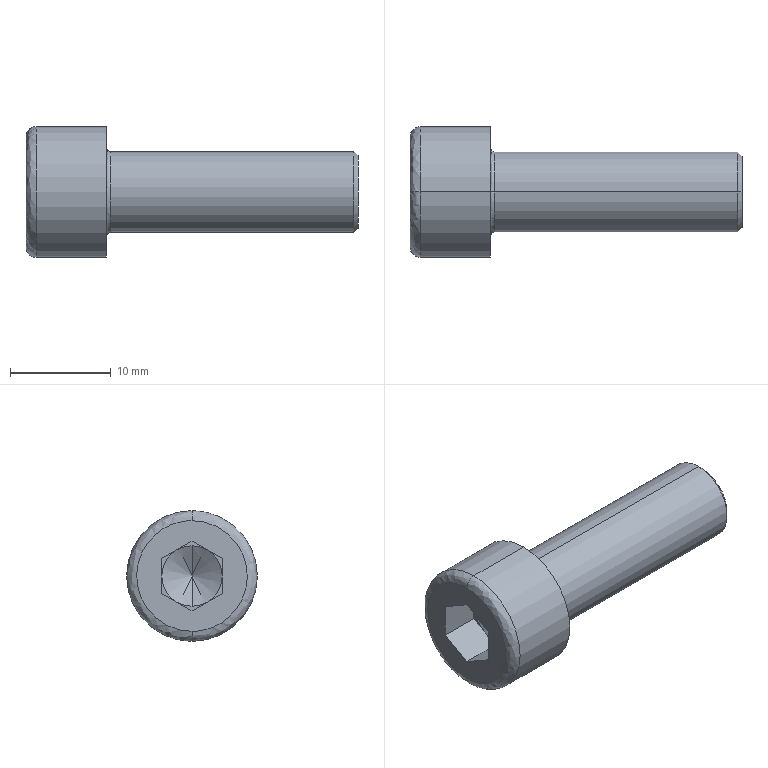Part | SolidWorks | features BaseBody 1 | 1 solid | 27 faces | box 33 x 13 x 13 mm | volume 2168 mm3 | plane 15 | spline 4 | cylinder 4 | cone 4 | commonest cylinder face diameters 8 x2 13 x2
STEP:
#1=CARTESIAN_POINT('',(8.,0.,4.4));
#2=VERTEX_POINT('',#1);
#3=CARTESIAN_POINT('',(8.,0.,-4.4));
#4=VERTEX_POINT('',#3);
#5=CARTESIAN_POINT('',(8.,0.,4.4));
#6=CARTESIAN_POINT('',(8.,0.2797,4.4));
#7=CARTESIAN_POINT('',(8.,0.6919,4.361));
#8=CARTESIAN_POINT('',(8.,1.16,4.249));
#9=CARTESIAN_POINT('',(8.,1.391,4.176));
#10=CARTESIAN_POINT('',(8.,1.489,4.141));
#11=CARTESIAN_POINT('',(8.,1.554,4.116));
#12=CARTESIAN_POINT('',(8.,1.585,4.105));
#13=CARTESIAN_POINT('',(8.,1.758,4.036));
#14=CARTESIAN_POINT('',(8.,1.96,3.944));
#15=CARTESIAN_POINT('',(8.,2.154,3.837));
#16=CARTESIAN_POINT('',(8.,2.282,3.763));
#17=CARTESIAN_POINT('',(8.,2.344,3.724));
#18=CARTESIAN_POINT('',(8.,2.662,3.517));
#19=CARTESIAN_POINT('',(8.,2.897,3.326));
#20=CARTESIAN_POINT('',(8.,3.219,3.004));
#21=CARTESIAN_POINT('',(8.,3.37,2.836));
#22=CARTESIAN_POINT('',(8.,3.509,2.656));
#23=CARTESIAN_POINT('',(8.,3.598,2.534));
#24=CARTESIAN_POINT('',(8.,3.642,2.47));
#25=CARTESIAN_POINT('',(8.,3.764,2.283));
#26=CARTESIAN_POINT('',(8.,3.876,2.092));
#27=CARTESIAN_POINT('',(8.,3.989,1.859));
#28=CARTESIAN_POINT('',(8.,4.042,1.74));
#29=CARTESIAN_POINT('',(8.,4.063,1.689));
#30=CARTESIAN_POINT('',(8.,4.077,1.654));
#31=CARTESIAN_POINT('',(8.,4.085,1.636));
#32=CARTESIAN_POINT('',(8.,4.297,1.1));
#33=CARTESIAN_POINT('',(8.,4.4,0.5592));
#34=CARTESIAN_POINT('',(8.,4.4,-0.2796));
#35=CARTESIAN_POINT('',(8.,4.361,-0.6917));
#36=CARTESIAN_POINT('',(8.,4.249,-1.16));
#37=CARTESIAN_POINT('',(8.,4.176,-1.391));
#38=CARTESIAN_POINT('',(8.,4.141,-1.489));
#39=CARTESIAN_POINT('',(8.,4.116,-1.554));
#40=CARTESIAN_POINT('',(8.,4.105,-1.585));
#41=CARTESIAN_POINT('',(8.,4.036,-1.758));
#42=CARTESIAN_POINT('',(8.,3.944,-1.96));
#43=CARTESIAN_POINT('',(8.,3.837,-2.154));
#44=CARTESIAN_POINT('',(8.,3.763,-2.282));
#45=CARTESIAN_POINT('',(8.,3.724,-2.344));
#46=CARTESIAN_POINT('',(8.,3.517,-2.662));
#47=CARTESIAN_POINT('',(8.,3.326,-2.897));
#48=CARTESIAN_POINT('',(8.,3.004,-3.219));
#49=CARTESIAN_POINT('',(8.,2.836,-3.37));
#50=CARTESIAN_POINT('',(8.,2.656,-3.509));
#51=CARTESIAN_POINT('',(8.,2.534,-3.598));
#52=CARTESIAN_POINT('',(8.,2.47,-3.642));
#53=CARTESIAN_POINT('',(8.,2.283,-3.764));
#54=CARTESIAN_POINT('',(8.,2.092,-3.876));
#55=CARTESIAN_POINT('',(8.,1.859,-3.989));
#56=CARTESIAN_POINT('',(8.,1.74,-4.042));
#57=CARTESIAN_POINT('',(8.,1.689,-4.063));
#58=CARTESIAN_POINT('',(8.,1.654,-4.077));
#59=CARTESIAN_POINT('',(8.,1.636,-4.085));
#60=CARTESIAN_POINT('',(8.,1.1,-4.297));
#61=CARTESIAN_POINT('',(8.,0.5597,-4.4));
#62=CARTESIAN_POINT('',(8.,0.,-4.4));
#63=B_SPLINE_CURVE_WITH_KNOTS('',3,(#5,#6,#7,#8,#9,#10,#11,#12,#13,#14,#15,#16,#17,#18,#19,#20,#21,#22,#23,#24,#25,#26,#27,#28,#29,#30,#31,#32,#33,#34,#35,#36,#37,#38,#39,#40,#41,#42,#43,#44,#45,#46,#47,#48,#49,#50,#51,#52,#53,#54,#55,#56,#57,#58,#59,#60,#61,#62),.UNSPECIFIED.,.F.,.F.,(4,1,1,1,2,2,1,2,2,2,1,2,2,1,1,1,2,2,2,1,1,1,2,2,1,2,2,2,1,2,2,1,1,1,2,2,4),(0.,0.0625,0.09375,0.1094,0.1172,0.125,0.1562,0.1719,0.1875,0.25,0.2812,0.2969,0.3125,0.3437,0.3594,0.3672,0.3711,0.375,0.5,0.5625,0.5937,0.6094,0.6172,0.625,0.6562,0.6719,0.6875,0.75,0.7812,0.7969,0.8125,0.8437,0.8594,0.8672,0.8711,0.875,1.),.UNSPECIFIED.);
#64=EDGE_CURVE('',#2,#4,#63,.T.);
#65=ORIENTED_EDGE('',*,*,#64,.F.);
#66=CARTESIAN_POINT('',(8.4,0.,4.));
#67=VERTEX_POINT('',#66);
#68=CARTESIAN_POINT('',(8.4,0.,4.4));
#69=DIRECTION('',(0.,-1.,0.));
#70=DIRECTION('',(0.,0.,1.));
#71=AXIS2_PLACEMENT_3D('',#68,#69,#70);
#72=CIRCLE('',#71,0.4);
#73=EDGE_CURVE('',#2,#67,#72,.T.);
#74=ORIENTED_EDGE('',*,*,#73,.T.);
#75=CARTESIAN_POINT('',(8.4,0.,-4.));
#76=VERTEX_POINT('',#75);
#77=CARTESIAN_POINT('',(8.4,0.,0.));
#78=DIRECTION('',(1.,0.,0.));
#79=DIRECTION('',(0.,0.,1.));
#80=AXIS2_PLACEMENT_3D('',#77,#78,#79);
#81=CIRCLE('',#80,4.);
#82=EDGE_CURVE('',#76,#67,#81,.T.);
#83=ORIENTED_EDGE('',*,*,#82,.F.);
#84=CARTESIAN_POINT('',(8.4,0.,-4.4));
#85=DIRECTION('',(0.,1.,0.));
#86=DIRECTION('',(0.,0.,-1.));
#87=AXIS2_PLACEMENT_3D('',#84,#85,#86);
#88=CIRCLE('',#87,0.4);
#89=EDGE_CURVE('',#4,#76,#88,.T.);
#90=ORIENTED_EDGE('',*,*,#89,.F.);
#91=EDGE_LOOP('',(#65,#74,#83,#90));
#92=FACE_OUTER_BOUND('',#91,.T.);
#93=CARTESIAN_POINT('',(8.,0.,-4.4));
#94=CARTESIAN_POINT('',(8.,8.8,-4.4));
#95=CARTESIAN_POINT('',(8.,8.8,4.4));
#96=CARTESIAN_POINT('',(8.,0.,4.4));
#97=CARTESIAN_POINT('',(8.,0.,-4.166));
#98=CARTESIAN_POINT('',(8.,8.331,-4.166));
#99=CARTESIAN_POINT('',(8.,8.331,4.166));
#100=CARTESIAN_POINT('',(8.,0.,4.166));
#101=CARTESIAN_POINT('',(8.166,0.,-4.));
#102=CARTESIAN_POINT('',(8.166,8.,-4.));
#103=CARTESIAN_POINT('',(8.166,8.,4.));
#104=CARTESIAN_POINT('',(8.166,0.,4.));
#105=CARTESIAN_POINT('',(8.4,0.,-4.));
#106=CARTESIAN_POINT('',(8.4,8.,-4.));
#107=CARTESIAN_POINT('',(8.4,8.,4.));
#108=CARTESIAN_POINT('',(8.4,0.,4.));
#109=(BOUNDED_SURFACE()B_SPLINE_SURFACE(3,3,((#93,#94,#95,#96),(#97,#98,#99,#100),(#101,#102,#103,#104),(#105,#106,#107,#108)),.UNSPECIFIED.,.F.,.F.,.T.)B_SPLINE_SURFACE_WITH_KNOTS((4,4),(4,4),(0.,1.),(0.,1.),.UNSPECIFIED.)GEOMETRIC_REPRESENTATION_ITEM()RATIONAL_B_SPLINE_SURFACE(((1.,0.3333,0.3333,1.),(0.8047,0.2682,0.2682,0.8047),(0.8047,0.2682,0.2682,0.8047),(1.,0.3333,0.3333,1.)))REPRESENTATION_ITEM('')SURFACE());
#110=ADVANCED_FACE('',(#92),#109,.F.);
#111=CARTESIAN_POINT('',(1.,0.,6.5));
#112=VERTEX_POINT('',#111);
#113=CARTESIAN_POINT('',(1.,0.,-6.5));
#114=VERTEX_POINT('',#113);
#115=CARTESIAN_POINT('',(1.,0.,0.));
#116=DIRECTION('',(1.,0.,0.));
#117=DIRECTION('',(0.,0.,1.));
#118=AXIS2_PLACEMENT_3D('',#115,#116,#117);
#119=CIRCLE('',#118,6.5);
#120=EDGE_CURVE('',#112,#114,#119,.T.);
#121=ORIENTED_EDGE('',*,*,#120,.F.);
#122=CARTESIAN_POINT('',(0.,0.,5.5));
#123=VERTEX_POINT('',#122);
#124=CARTESIAN_POINT('',(1.,0.,5.5));
#125=DIRECTION('',(0.,-1.,0.));
#126=DIRECTION('',(0.,0.,1.));
#127=AXIS2_PLACEMENT_3D('',#124,#125,#126);
#128=CIRCLE('',#127,1.);
#129=EDGE_CURVE('',#112,#123,#128,.T.);
#130=ORIENTED_EDGE('',*,*,#129,.T.);
#131=CARTESIAN_POINT('',(0.,0.,-5.5));
#132=VERTEX_POINT('',#131);
#133=CARTESIAN_POINT('',(0.,0.,5.5));
#134=CARTESIAN_POINT('',(0.,-11.,5.5));
#135=CARTESIAN_POINT('',(0.,-11.,-5.5));
#136=CARTESIAN_POINT('',(0.,0.,-5.5));
#137=(BOUNDED_CURVE()B_SPLINE_CURVE(3,(#133,#134,#135,#136),.UNSPECIFIED.,.F.,.F.)B_SPLINE_CURVE_WITH_KNOTS((4,4),(0.,1.),.UNSPECIFIED.)CURVE()GEOMETRIC_REPRESENTATION_ITEM()RATIONAL_B_SPLINE_CURVE((1.,0.3333,0.3333,1.))REPRESENTATION_ITEM(''));
#138=EDGE_CURVE('',#123,#132,#137,.T.);
#139=ORIENTED_EDGE('',*,*,#138,.T.);
#140=CARTESIAN_POINT('',(1.,0.,-5.5));
#141=DIRECTION('',(0.,1.,0.));
#142=DIRECTION('',(0.,0.,-1.));
#143=AXIS2_PLACEMENT_3D('',#140,#141,#142);
#144=CIRCLE('',#143,1.);
#145=EDGE_CURVE('',#114,#132,#144,.T.);
#146=ORIENTED_EDGE('',*,*,#145,.F.);
#147=EDGE_LOOP('',(#121,#130,#139,#146));
#148=FACE_OUTER_BOUND('',#147,.T.);
#149=CARTESIAN_POINT('',(1.,0.,6.5));
#150=CARTESIAN_POINT('',(1.,-13.,6.5));
#151=CARTESIAN_POINT('',(1.,-13.,-6.5));
#152=CARTESIAN_POINT('',(1.,0.,-6.5));
#153=CARTESIAN_POINT('',(0.4142,0.,6.5));
#154=CARTESIAN_POINT('',(0.4142,-13.,6.5));
#155=CARTESIAN_POINT('',(0.4142,-13.,-6.5));
#156=CARTESIAN_POINT('',(0.4142,0.,-6.5));
#157=CARTESIAN_POINT('',(0.,0.,6.086));
#158=CARTESIAN_POINT('',(0.,-12.172,6.086));
#159=CARTESIAN_POINT('',(0.,-12.172,-6.086));
#160=CARTESIAN_POINT('',(0.,0.,-6.086));
#161=CARTESIAN_POINT('',(0.,0.,5.5));
#162=CARTESIAN_POINT('',(0.,-11.,5.5));
#163=CARTESIAN_POINT('',(0.,-11.,-5.5));
#164=CARTESIAN_POINT('',(0.,0.,-5.5));
#165=(BOUNDED_SURFACE()B_SPLINE_SURFACE(3,3,((#149,#150,#151,#152),(#153,#154,#155,#156),(#157,#158,#159,#160),(#161,#162,#163,#164)),.UNSPECIFIED.,.F.,.F.,.T.)B_SPLINE_SURFACE_WITH_KNOTS((4,4),(4,4),(0.,1.),(0.,1.),.UNSPECIFIED.)GEOMETRIC_REPRESENTATION_ITEM()RATIONAL_B_SPLINE_SURFACE(((1.,0.3333,0.3333,1.),(0.8047,0.2682,0.2682,0.8047),(0.8047,0.2682,0.2682,0.8047),(1.,0.3333,0.3333,1.)))REPRESENTATION_ITEM('')SURFACE());
#166=ADVANCED_FACE('',(#148),#165,.T.);
#167=CARTESIAN_POINT('',(32.6,0.,4.));
#168=VERTEX_POINT('',#167);
#169=CARTESIAN_POINT('',(32.6,0.,-4.));
#170=VERTEX_POINT('',#169);
#171=CARTESIAN_POINT('',(32.6,0.,0.));
#172=DIRECTION('',(-1.,0.,0.));
#173=DIRECTION('',(0.,0.,1.));
#174=AXIS2_PLACEMENT_3D('',#171,#172,#173);
#175=CIRCLE('',#174,4.);
#176=EDGE_CURVE('',#168,#170,#175,.T.);
#177=ORIENTED_EDGE('',*,*,#176,.T.);
#178=CARTESIAN_POINT('',(33.,0.,-4.));
#179=DIRECTION('',(-1.,0.,0.));
#180=VECTOR('',#179,1000.);
#181=LINE('',#178,#180);
#182=EDGE_CURVE('',#170,#76,#181,.T.);
#183=ORIENTED_EDGE('',*,*,#182,.T.);
#184=ORIENTED_EDGE('',*,*,#82,.T.);
#185=CARTESIAN_POINT('',(33.,0.,4.));
#186=DIRECTION('',(-1.,0.,0.));
#187=VECTOR('',#186,1000.);
#188=LINE('',#185,#187);
#189=EDGE_CURVE('',#168,#67,#188,.T.);
#190=ORIENTED_EDGE('',*,*,#189,.F.);
#191=EDGE_LOOP('',(#177,#183,#184,#190));
#192=FACE_OUTER_BOUND('',#191,.T.);
#193=CARTESIAN_POINT('',(33.,0.,0.));
#194=DIRECTION('',(-1.,0.,0.));
#195=DIRECTION('',(0.,0.,1.));
#196=AXIS2_PLACEMENT_3D('',#193,#194,#195);
#197=CYLINDRICAL_SURFACE('',#196,4.);
#198=ADVANCED_FACE('',(#192),#197,.T.);
#199=CARTESIAN_POINT('',(33.,0.,3.6));
#200=VERTEX_POINT('',#199);
#201=CARTESIAN_POINT('',(33.,0.,-3.6));
#202=VERTEX_POINT('',#201);
#203=CARTESIAN_POINT('',(33.,0.,0.));
#204=DIRECTION('',(-1.,0.,0.));
#205=DIRECTION('',(0.,0.,1.));
#206=AXIS2_PLACEMENT_3D('',#203,#204,#205);
#207=CIRCLE('',#206,3.6);
#208=EDGE_CURVE('',#200,#202,#207,.T.);
#209=ORIENTED_EDGE('',*,*,#208,.T.);
#210=CARTESIAN_POINT('',(32.6,0.,-4.));
#211=DIRECTION('',(-0.7071,0.,-0.7071));
#212=VECTOR('',#211,1000.);
#213=LINE('',#210,#212);
#214=EDGE_CURVE('',#202,#170,#213,.T.);
#215=ORIENTED_EDGE('',*,*,#214,.T.);
#216=ORIENTED_EDGE('',*,*,#176,.F.);
#217=CARTESIAN_POINT('',(32.6,0.,4.));
#218=DIRECTION('',(-0.7071,0.,0.7071));
#219=VECTOR('',#218,1000.);
#220=LINE('',#217,#219);
#221=EDGE_CURVE('',#200,#168,#220,.T.);
#222=ORIENTED_EDGE('',*,*,#221,.F.);
#223=EDGE_LOOP('',(#209,#215,#216,#222));
#224=FACE_OUTER_BOUND('',#223,.T.);
#225=CARTESIAN_POINT('',(32.6,0.,0.));
#226=DIRECTION('',(-1.,0.,0.));
#227=DIRECTION('',(0.,0.,1.));
#228=AXIS2_PLACEMENT_3D('',#225,#226,#227);
#229=CONICAL_SURFACE('',#228,4.,0.7854);
#230=ADVANCED_FACE('',(#224),#229,.T.);
#231=CARTESIAN_POINT('',(8.,0.,-6.5));
#232=VERTEX_POINT('',#231);
#233=CARTESIAN_POINT('',(8.,0.,6.5));
#234=VERTEX_POINT('',#233);
#235=CARTESIAN_POINT('',(8.,0.,0.));
#236=DIRECTION('',(1.,0.,0.));
#237=DIRECTION('',(0.,0.,1.));
#238=AXIS2_PLACEMENT_3D('',#235,#236,#237);
#239=CIRCLE('',#238,6.5);
#240=EDGE_CURVE('',#232,#234,#239,.T.);
#241=ORIENTED_EDGE('',*,*,#240,.F.);
#242=CARTESIAN_POINT('',(8.,0.,-6.5));
#243=DIRECTION('',(-1.,0.,0.));
#244=VECTOR('',#243,1000.);
#245=LINE('',#242,#244);
#246=EDGE_CURVE('',#232,#114,#245,.T.);
#247=ORIENTED_EDGE('',*,*,#246,.T.);
#248=CARTESIAN_POINT('',(1.,0.,0.));
#249=DIRECTION('',(1.,0.,0.));
#250=DIRECTION('',(0.,0.,1.));
#251=AXIS2_PLACEMENT_3D('',#248,#249,#250);
#252=CIRCLE('',#251,6.5);
#253=EDGE_CURVE('',#114,#112,#252,.T.);
#254=ORIENTED_EDGE('',*,*,#253,.T.);
#255=CARTESIAN_POINT('',(8.,0.,6.5));
#256=DIRECTION('',(-1.,0.,0.));
#257=VECTOR('',#256,1000.);
#258=LINE('',#255,#257);
#259=EDGE_CURVE('',#234,#112,#258,.T.);
#260=ORIENTED_EDGE('',*,*,#259,.F.);
#261=EDGE_LOOP('',(#241,#247,#254,#260));
#262=FACE_OUTER_BOUND('',#261,.T.);
#263=CARTESIAN_POINT('',(8.,0.,0.));
#264=DIRECTION('',(-1.,0.,0.));
#265=DIRECTION('',(0.,0.,1.));
#266=AXIS2_PLACEMENT_3D('',#263,#264,#265);
#267=CYLINDRICAL_SURFACE('',#266,6.5);
#268=ADVANCED_FACE('',(#262),#267,.T.);
#269=CARTESIAN_POINT('',(5.732,0.,0.));
#270=VERTEX_POINT('',#269);
#271=CARTESIAN_POINT('',(4.,0.,3.));
#272=VERTEX_POINT('',#271);
#273=CARTESIAN_POINT('',(4.,0.,3.));
#274=DIRECTION('',(-0.5,0.,0.866));
#275=VECTOR('',#274,1000.);
#276=LINE('',#273,#275);
#277=EDGE_CURVE('',#270,#272,#276,.T.);
#278=ORIENTED_EDGE('',*,*,#277,.F.);
#279=CARTESIAN_POINT('',(4.,0.,-3.));
#280=VERTEX_POINT('',#279);
#281=CARTESIAN_POINT('',(4.,0.,-3.));
#282=DIRECTION('',(-0.5,0.,-0.866));
#283=VECTOR('',#282,1000.);
#284=LINE('',#281,#283);
#285=EDGE_CURVE('',#270,#280,#284,.T.);
#286=ORIENTED_EDGE('',*,*,#285,.T.);
#287=CARTESIAN_POINT('',(4.,-1.5,-2.598));
#288=VERTEX_POINT('',#287);
#289=CARTESIAN_POINT('',(4.,0.,0.));
#290=DIRECTION('',(1.,0.,0.));
#291=DIRECTION('',(0.,0.,1.));
#292=AXIS2_PLACEMENT_3D('',#289,#290,#291);
#293=CIRCLE('',#292,3.);
#294=EDGE_CURVE('',#288,#280,#293,.T.);
#295=ORIENTED_EDGE('',*,*,#294,.F.);
#296=CARTESIAN_POINT('',(4.,-3.,0.));
#297=VERTEX_POINT('',#296);
#298=CARTESIAN_POINT('',(4.,0.,0.));
#299=DIRECTION('',(-1.,0.,0.));
#300=DIRECTION('',(0.,0.,1.));
#301=AXIS2_PLACEMENT_3D('',#298,#299,#300);
#302=CIRCLE('',#301,3.);
#303=EDGE_CURVE('',#288,#297,#302,.T.);
#304=ORIENTED_EDGE('',*,*,#303,.T.);
#305=CARTESIAN_POINT('',(4.,-1.5,2.598));
#306=VERTEX_POINT('',#305);
#307=CARTESIAN_POINT('',(4.,0.,0.));
#308=DIRECTION('',(1.,0.,0.));
#309=DIRECTION('',(0.,0.,1.));
#310=AXIS2_PLACEMENT_3D('',#307,#308,#309);
#311=CIRCLE('',#310,3.);
#312=EDGE_CURVE('',#306,#297,#311,.T.);
#313=ORIENTED_EDGE('',*,*,#312,.F.);
#314=CARTESIAN_POINT('',(4.,0.,0.));
#315=DIRECTION('',(1.,0.,0.));
#316=DIRECTION('',(0.,0.,1.));
#317=AXIS2_PLACEMENT_3D('',#314,#315,#316);
#318=CIRCLE('',#317,3.);
#319=EDGE_CURVE('',#272,#306,#318,.T.);
#320=ORIENTED_EDGE('',*,*,#319,.F.);
#321=EDGE_LOOP('',(#278,#286,#295,#304,#313,#320));
#322=FACE_OUTER_BOUND('',#321,.T.);
#323=CARTESIAN_POINT('',(4.,0.,0.));
#324=DIRECTION('',(-1.,0.,0.));
#325=DIRECTION('',(0.,0.,1.));
#326=AXIS2_PLACEMENT_3D('',#323,#324,#325);
#327=CONICAL_SURFACE('',#326,3.,1.047);
#328=ADVANCED_FACE('',(#322),#327,.F.);
#329=ORIENTED_EDGE('',*,*,#182,.F.);
#330=CARTESIAN_POINT('',(32.6,0.,0.));
#331=DIRECTION('',(-1.,0.,0.));
#332=DIRECTION('',(0.,0.,1.));
#333=AXIS2_PLACEMENT_3D('',#330,#331,#332);
#334=CIRCLE('',#333,4.);
#335=EDGE_CURVE('',#170,#168,#334,.T.);
#336=ORIENTED_EDGE('',*,*,#335,.T.);
#337=ORIENTED_EDGE('',*,*,#189,.T.);
#338=CARTESIAN_POINT('',(8.4,0.,0.));
#339=DIRECTION('',(1.,0.,0.));
#340=DIRECTION('',(0.,0.,1.));
#341=AXIS2_PLACEMENT_3D('',#338,#339,#340);
#342=CIRCLE('',#341,4.);
#343=EDGE_CURVE('',#67,#76,#342,.T.);
#344=ORIENTED_EDGE('',*,*,#343,.T.);
#345=EDGE_LOOP('',(#329,#336,#337,#344));
#346=FACE_OUTER_BOUND('',#345,.T.);
#347=CARTESIAN_POINT('',(33.,0.,0.));
#348=DIRECTION('',(-1.,0.,0.));
#349=DIRECTION('',(0.,0.,1.));
#350=AXIS2_PLACEMENT_3D('',#347,#348,#349);
#351=CYLINDRICAL_SURFACE('',#350,4.);
#352=ADVANCED_FACE('',(#346),#351,.T.);
#353=ORIENTED_EDGE('',*,*,#73,.F.);
#354=CARTESIAN_POINT('',(8.,0.,-4.4));
#355=CARTESIAN_POINT('',(8.,-0.2797,-4.4));
#356=CARTESIAN_POINT('',(8.,-0.6919,-4.361));
#357=CARTESIAN_POINT('',(8.,-1.16,-4.249));
#358=CARTESIAN_POINT('',(8.,-1.391,-4.176));
#359=CARTESIAN_POINT('',(8.,-1.489,-4.141));
#360=CARTESIAN_POINT('',(8.,-1.554,-4.116));
#361=CARTESIAN_POINT('',(8.,-1.585,-4.105));
#362=CARTESIAN_POINT('',(8.,-1.758,-4.036));
#363=CARTESIAN_POINT('',(8.,-1.96,-3.944));
#364=CARTESIAN_POINT('',(8.,-2.154,-3.837));
#365=CARTESIAN_POINT('',(8.,-2.282,-3.763));
#366=CARTESIAN_POINT('',(8.,-2.344,-3.724));
#367=CARTESIAN_POINT('',(8.,-2.662,-3.517));
#368=CARTESIAN_POINT('',(8.,-2.897,-3.326));
#369=CARTESIAN_POINT('',(8.,-3.219,-3.004));
#370=CARTESIAN_POINT('',(8.,-3.37,-2.836));
#371=CARTESIAN_POINT('',(8.,-3.509,-2.656));
#372=CARTESIAN_POINT('',(8.,-3.598,-2.534));
#373=CARTESIAN_POINT('',(8.,-3.642,-2.47));
#374=CARTESIAN_POINT('',(8.,-3.764,-2.283));
#375=CARTESIAN_POINT('',(8.,-3.876,-2.092));
#376=CARTESIAN_POINT('',(8.,-3.989,-1.859));
#377=CARTESIAN_POINT('',(8.,-4.042,-1.74));
#378=CARTESIAN_POINT('',(8.,-4.063,-1.689));
#379=CARTESIAN_POINT('',(8.,-4.077,-1.654));
#380=CARTESIAN_POINT('',(8.,-4.085,-1.636));
#381=CARTESIAN_POINT('',(8.,-4.297,-1.1));
#382=CARTESIAN_POINT('',(8.,-4.4,-0.5592));
#383=CARTESIAN_POINT('',(8.,-4.4,0.2796));
#384=CARTESIAN_POINT('',(8.,-4.361,0.6917));
#385=CARTESIAN_POINT('',(8.,-4.249,1.16));
#386=CARTESIAN_POINT('',(8.,-4.176,1.391));
#387=CARTESIAN_POINT('',(8.,-4.141,1.489));
#388=CARTESIAN_POINT('',(8.,-4.116,1.554));
#389=CARTESIAN_POINT('',(8.,-4.105,1.585));
#390=CARTESIAN_POINT('',(8.,-4.036,1.758));
#391=CARTESIAN_POINT('',(8.,-3.944,1.96));
#392=CARTESIAN_POINT('',(8.,-3.837,2.154));
#393=CARTESIAN_POINT('',(8.,-3.763,2.282));
#394=CARTESIAN_POINT('',(8.,-3.724,2.344));
#395=CARTESIAN_POINT('',(8.,-3.517,2.662));
#396=CARTESIAN_POINT('',(8.,-3.326,2.897));
#397=CARTESIAN_POINT('',(8.,-3.004,3.219));
#398=CARTESIAN_POINT('',(8.,-2.836,3.37));
#399=CARTESIAN_POINT('',(8.,-2.656,3.509));
#400=CARTESIAN_POINT('',(8.,-2.534,3.598));
#401=CARTESIAN_POINT('',(8.,-2.47,3.642));
#402=CARTESIAN_POINT('',(8.,-2.283,3.764));
#403=CARTESIAN_POINT('',(8.,-2.092,3.876));
#404=CARTESIAN_POINT('',(8.,-1.859,3.989));
#405=CARTESIAN_POINT('',(8.,-1.74,4.042));
#406=CARTESIAN_POINT('',(8.,-1.689,4.063));
#407=CARTESIAN_POINT('',(8.,-1.654,4.077));
#408=CARTESIAN_POINT('',(8.,-1.636,4.085));
#409=CARTESIAN_POINT('',(8.,-1.1,4.297));
#410=CARTESIAN_POINT('',(8.,-0.5597,4.4));
#411=CARTESIAN_POINT('',(8.,0.,4.4));
#412=B_SPLINE_CURVE_WITH_KNOTS('',3,(#354,#355,#356,#357,#358,#359,#360,#361,#362,#363,#364,#365,#366,#367,#368,#369,#370,#371,#372,#373,#374,#375,#376,#377,#378,#379,#380,#381,#382,#383,#384,#385,#386,#387,#388,#389,#390,#391,#392,#393,#394,#395,#396,#397,#398,#399,#400,#401,#402,#403,#404,#405,#406,#407,#408,#409,#410,#411),.UNSPECIFIED.,.F.,.F.,(4,1,1,1,2,2,1,2,2,2,1,2,2,1,1,1,2,2,2,1,1,1,2,2,1,2,2,2,1,2,2,1,1,1,2,2,4),(0.,0.0625,0.09375,0.1094,0.1172,0.125,0.1563,0.1719,0.1875,0.25,0.2813,0.2969,0.3125,0.3438,0.3594,0.3672,0.3711,0.375,0.5,0.5625,0.5938,0.6094,0.6172,0.625,0.6563,0.6719,0.6875,0.75,0.7813,0.7969,0.8125,0.8438,0.8594,0.8672,0.8711,0.875,1.),.UNSPECIFIED.);
#413=EDGE_CURVE('',#4,#2,#412,.T.);
#414=ORIENTED_EDGE('',*,*,#413,.F.);
#415=ORIENTED_EDGE('',*,*,#89,.T.);
#416=ORIENTED_EDGE('',*,*,#343,.F.);
#417=EDGE_LOOP('',(#353,#414,#415,#416));
#418=FACE_OUTER_BOUND('',#417,.T.);
#419=CARTESIAN_POINT('',(8.,0.,4.4));
#420=CARTESIAN_POINT('',(8.,-8.8,4.4));
#421=CARTESIAN_POINT('',(8.,-8.8,-4.4));
#422=CARTESIAN_POINT('',(8.,0.,-4.4));
#423=CARTESIAN_POINT('',(8.,0.,4.166));
#424=CARTESIAN_POINT('',(8.,-8.331,4.166));
#425=CARTESIAN_POINT('',(8.,-8.331,-4.166));
#426=CARTESIAN_POINT('',(8.,0.,-4.166));
#427=CARTESIAN_POINT('',(8.166,0.,4.));
#428=CARTESIAN_POINT('',(8.166,-8.,4.));
#429=CARTESIAN_POINT('',(8.166,-8.,-4.));
#430=CARTESIAN_POINT('',(8.166,0.,-4.));
#431=CARTESIAN_POINT('',(8.4,0.,4.));
#432=CARTESIAN_POINT('',(8.4,-8.,4.));
#433=CARTESIAN_POINT('',(8.4,-8.,-4.));
#434=CARTESIAN_POINT('',(8.4,0.,-4.));
#435=(BOUNDED_SURFACE()B_SPLINE_SURFACE(3,3,((#419,#420,#421,#422),(#423,#424,#425,#426),(#427,#428,#429,#430),(#431,#432,#433,#434)),.UNSPECIFIED.,.F.,.F.,.F.)B_SPLINE_SURFACE_WITH_KNOTS((4,4),(4,4),(0.,1.),(0.,1.),.UNSPECIFIED.)GEOMETRIC_REPRESENTATION_ITEM()RATIONAL_B_SPLINE_SURFACE(((1.,0.3333,0.3333,1.),(0.8047,0.2682,0.2682,0.8047),(0.8047,0.2682,0.2682,0.8047),(1.,0.3333,0.3333,1.)))REPRESENTATION_ITEM('')SURFACE());
#436=ADVANCED_FACE('',(#418),#435,.F.);
#437=ORIENTED_EDGE('',*,*,#214,.F.);
#438=CARTESIAN_POINT('',(33.,0.,0.));
#439=DIRECTION('',(-1.,0.,0.));
#440=DIRECTION('',(0.,0.,1.));
#441=AXIS2_PLACEMENT_3D('',#438,#439,#440);
#442=CIRCLE('',#441,3.6);
#443=EDGE_CURVE('',#202,#200,#442,.T.);
#444=ORIENTED_EDGE('',*,*,#443,.T.);
#445=ORIENTED_EDGE('',*,*,#221,.T.);
#446=ORIENTED_EDGE('',*,*,#335,.F.);
#447=EDGE_LOOP('',(#437,#444,#445,#446));
#448=FACE_OUTER_BOUND('',#447,.T.);
#449=CARTESIAN_POINT('',(32.6,0.,0.));
#450=DIRECTION('',(-1.,0.,0.));
#451=DIRECTION('',(0.,0.,1.));
#452=AXIS2_PLACEMENT_3D('',#449,#450,#451);
#453=CONICAL_SURFACE('',#452,4.,0.7854);
#454=ADVANCED_FACE('',(#448),#453,.T.);
#455=CARTESIAN_POINT('',(8.,0.,0.));
#456=DIRECTION('',(1.,0.,0.));
#457=DIRECTION('',(0.,0.,1.));
#458=AXIS2_PLACEMENT_3D('',#455,#456,#457);
#459=CIRCLE('',#458,6.5);
#460=EDGE_CURVE('',#234,#232,#459,.T.);
#461=ORIENTED_EDGE('',*,*,#460,.T.);
#462=ORIENTED_EDGE('',*,*,#240,.T.);
#463=EDGE_LOOP('',(#461,#462));
#464=FACE_OUTER_BOUND('',#463,.T.);
#465=ORIENTED_EDGE('',*,*,#413,.T.);
#466=ORIENTED_EDGE('',*,*,#64,.T.);
#467=EDGE_LOOP('',(#465,#466));
#468=FACE_BOUND('',#467,.T.);
#469=CARTESIAN_POINT('',(8.,0.,0.));
#470=DIRECTION('',(1.,0.,0.));
#471=DIRECTION('',(0.,0.,-1.));
#472=AXIS2_PLACEMENT_3D('',#469,#470,#471);
#473=PLANE('',#472);
#474=ADVANCED_FACE('',(#464,#468),#473,.T.);
#475=ORIENTED_EDGE('',*,*,#208,.F.);
#476=ORIENTED_EDGE('',*,*,#443,.F.);
#477=EDGE_LOOP('',(#475,#476));
#478=FACE_OUTER_BOUND('',#477,.T.);
#479=CARTESIAN_POINT('',(33.,0.,0.));
#480=DIRECTION('',(1.,0.,0.));
#481=DIRECTION('',(0.,0.,-1.));
#482=AXIS2_PLACEMENT_3D('',#479,#480,#481);
#483=PLANE('',#482);
#484=ADVANCED_FACE('',(#478),#483,.T.);
#485=ORIENTED_EDGE('',*,*,#246,.F.);
#486=ORIENTED_EDGE('',*,*,#460,.F.);
#487=ORIENTED_EDGE('',*,*,#259,.T.);
#488=ORIENTED_EDGE('',*,*,#120,.T.);
#489=EDGE_LOOP('',(#485,#486,#487,#488));
#490=FACE_OUTER_BOUND('',#489,.T.);
#491=CARTESIAN_POINT('',(8.,0.,0.));
#492=DIRECTION('',(-1.,0.,0.));
#493=DIRECTION('',(0.,0.,1.));
#494=AXIS2_PLACEMENT_3D('',#491,#492,#493);
#495=CYLINDRICAL_SURFACE('',#494,6.5);
#496=ADVANCED_FACE('',(#490),#495,.T.);
#497=ORIENTED_EDGE('',*,*,#129,.F.);
#498=ORIENTED_EDGE('',*,*,#253,.F.);
#499=ORIENTED_EDGE('',*,*,#145,.T.);
#500=CARTESIAN_POINT('',(0.,0.,-5.5));
#501=CARTESIAN_POINT('',(0.,11.,-5.5));
#502=CARTESIAN_POINT('',(0.,11.,5.5));
#503=CARTESIAN_POINT('',(0.,0.,5.5));
#504=(BOUNDED_CURVE()B_SPLINE_CURVE(3,(#500,#501,#502,#503),.UNSPECIFIED.,.F.,.F.)B_SPLINE_CURVE_WITH_KNOTS((4,4),(0.,1.),.UNSPECIFIED.)CURVE()GEOMETRIC_REPRESENTATION_ITEM()RATIONAL_B_SPLINE_CURVE((1.,0.3333,0.3333,1.))REPRESENTATION_ITEM(''));
#505=EDGE_CURVE('',#132,#123,#504,.T.);
#506=ORIENTED_EDGE('',*,*,#505,.T.);
#507=EDGE_LOOP('',(#497,#498,#499,#506));
#508=FACE_OUTER_BOUND('',#507,.T.);
#509=CARTESIAN_POINT('',(1.,0.,-6.5));
#510=CARTESIAN_POINT('',(1.,13.,-6.5));
#511=CARTESIAN_POINT('',(1.,13.,6.5));
#512=CARTESIAN_POINT('',(1.,0.,6.5));
#513=CARTESIAN_POINT('',(0.4142,0.,-6.5));
#514=CARTESIAN_POINT('',(0.4142,13.,-6.5));
#515=CARTESIAN_POINT('',(0.4142,13.,6.5));
#516=CARTESIAN_POINT('',(0.4142,0.,6.5));
#517=CARTESIAN_POINT('',(0.,0.,-6.086));
#518=CARTESIAN_POINT('',(0.,12.172,-6.086));
#519=CARTESIAN_POINT('',(0.,12.172,6.086));
#520=CARTESIAN_POINT('',(0.,0.,6.086));
#521=CARTESIAN_POINT('',(0.,0.,-5.5));
#522=CARTESIAN_POINT('',(0.,11.,-5.5));
#523=CARTESIAN_POINT('',(0.,11.,5.5));
#524=CARTESIAN_POINT('',(0.,0.,5.5));
#525=(BOUNDED_SURFACE()B_SPLINE_SURFACE(3,3,((#509,#510,#511,#512),(#513,#514,#515,#516),(#517,#518,#519,#520),(#521,#522,#523,#524)),.UNSPECIFIED.,.F.,.F.,.T.)B_SPLINE_SURFACE_WITH_KNOTS((4,4),(4,4),(0.,1.),(0.,1.),.UNSPECIFIED.)GEOMETRIC_REPRESENTATION_ITEM()RATIONAL_B_SPLINE_SURFACE(((1.,0.3333,0.3333,1.),(0.8047,0.2682,0.2682,0.8047),(0.8047,0.2682,0.2682,0.8047),(1.,0.3333,0.3333,1.)))REPRESENTATION_ITEM('')SURFACE());
#526=ADVANCED_FACE('',(#508),#525,.T.);
#527=CARTESIAN_POINT('',(0.,3.,1.732));
#528=VERTEX_POINT('',#527);
#529=CARTESIAN_POINT('',(0.,3.,-1.732));
#530=VERTEX_POINT('',#529);
#531=CARTESIAN_POINT('',(0.,3.,0.));
#532=DIRECTION('',(0.,0.,-1.));
#533=VECTOR('',#532,1000.);
#534=LINE('',#531,#533);
#535=EDGE_CURVE('',#528,#530,#534,.T.);
#536=ORIENTED_EDGE('',*,*,#535,.F.);
#537=CARTESIAN_POINT('',(0.,0.,3.464));
#538=VERTEX_POINT('',#537);
#539=CARTESIAN_POINT('',(0.,0.,3.464));
#540=DIRECTION('',(0.,0.866,-0.5));
#541=VECTOR('',#540,1000.);
#542=LINE('',#539,#541);
#543=EDGE_CURVE('',#538,#528,#542,.T.);
#544=ORIENTED_EDGE('',*,*,#543,.F.);
#545=CARTESIAN_POINT('',(0.,-3.,1.732));
#546=VERTEX_POINT('',#545);
#547=CARTESIAN_POINT('',(0.,-3.,1.732));
#548=DIRECTION('',(0.,0.866,0.5));
#549=VECTOR('',#548,1000.);
#550=LINE('',#547,#549);
#551=EDGE_CURVE('',#546,#538,#550,.T.);
#552=ORIENTED_EDGE('',*,*,#551,.F.);
#553=CARTESIAN_POINT('',(0.,-3.,-1.732));
#554=VERTEX_POINT('',#553);
#555=CARTESIAN_POINT('',(0.,-3.,0.));
#556=DIRECTION('',(0.,0.,1.));
#557=VECTOR('',#556,1000.);
#558=LINE('',#555,#557);
#559=EDGE_CURVE('',#554,#546,#558,.T.);
#560=ORIENTED_EDGE('',*,*,#559,.F.);
#561=CARTESIAN_POINT('',(0.,0.,-3.464));
#562=VERTEX_POINT('',#561);
#563=CARTESIAN_POINT('',(0.,0.,-3.464));
#564=DIRECTION('',(0.,-0.866,0.5));
#565=VECTOR('',#564,1000.);
#566=LINE('',#563,#565);
#567=EDGE_CURVE('',#562,#554,#566,.T.);
#568=ORIENTED_EDGE('',*,*,#567,.F.);
#569=CARTESIAN_POINT('',(0.,3.,-1.732));
#570=DIRECTION('',(0.,-0.866,-0.5));
#571=VECTOR('',#570,1000.);
#572=LINE('',#569,#571);
#573=EDGE_CURVE('',#530,#562,#572,.T.);
#574=ORIENTED_EDGE('',*,*,#573,.F.);
#575=EDGE_LOOP('',(#536,#544,#552,#560,#568,#574));
#576=FACE_BOUND('',#575,.T.);
#577=ORIENTED_EDGE('',*,*,#505,.F.);
#578=ORIENTED_EDGE('',*,*,#138,.F.);
#579=EDGE_LOOP('',(#577,#578));
#580=FACE_OUTER_BOUND('',#579,.T.);
#581=CARTESIAN_POINT('',(0.,0.,0.));
#582=DIRECTION('',(1.,0.,0.));
#583=DIRECTION('',(0.,0.,-1.));
#584=AXIS2_PLACEMENT_3D('',#581,#582,#583);
#585=PLANE('',#584);
#586=ADVANCED_FACE('',(#576,#580),#585,.F.);
#587=CARTESIAN_POINT('',(4.,0.,-3.464));
#588=VERTEX_POINT('',#587);
#589=CARTESIAN_POINT('',(4.,0.,-3.464));
#590=DIRECTION('',(1.,0.,0.));
#591=VECTOR('',#590,1000.);
#592=LINE('',#589,#591);
#593=EDGE_CURVE('',#562,#588,#592,.T.);
#594=ORIENTED_EDGE('',*,*,#593,.T.);
#595=CARTESIAN_POINT('',(4.,1.5,-2.598));
#596=VERTEX_POINT('',#595);
#597=CARTESIAN_POINT('',(4.,0.,-3.464));
#598=DIRECTION('',(0.,0.866,0.5));
#599=VECTOR('',#598,1000.);
#600=LINE('',#597,#599);
#601=EDGE_CURVE('',#588,#596,#600,.T.);
#602=ORIENTED_EDGE('',*,*,#601,.T.);
#603=CARTESIAN_POINT('',(4.,3.,-1.732));
#604=VERTEX_POINT('',#603);
#605=CARTESIAN_POINT('',(4.,1.5,-2.598));
#606=DIRECTION('',(0.,0.866,0.5));
#607=VECTOR('',#606,1000.);
#608=LINE('',#605,#607);
#609=EDGE_CURVE('',#596,#604,#608,.T.);
#610=ORIENTED_EDGE('',*,*,#609,.T.);
#611=CARTESIAN_POINT('',(4.,3.,-1.732));
#612=DIRECTION('',(-1.,0.,0.));
#613=VECTOR('',#612,1000.);
#614=LINE('',#611,#613);
#615=EDGE_CURVE('',#604,#530,#614,.T.);
#616=ORIENTED_EDGE('',*,*,#615,.T.);
#617=ORIENTED_EDGE('',*,*,#573,.T.);
#618=EDGE_LOOP('',(#594,#602,#610,#616,#617));
#619=FACE_OUTER_BOUND('',#618,.T.);
#620=CARTESIAN_POINT('',(4.,0.,-3.464));
#621=DIRECTION('',(0.,-0.5,0.866));
#622=DIRECTION('',(0.,-0.866,-0.5));
#623=AXIS2_PLACEMENT_3D('',#620,#621,#622);
#624=PLANE('',#623);
#625=ADVANCED_FACE('',(#619),#624,.T.);
#626=ORIENTED_EDGE('',*,*,#615,.F.);
#627=CARTESIAN_POINT('',(4.,3.,0.));
#628=VERTEX_POINT('',#627);
#629=CARTESIAN_POINT('',(4.,3.,-3.464));
#630=DIRECTION('',(0.,0.,1.));
#631=VECTOR('',#630,1000.);
#632=LINE('',#629,#631);
#633=EDGE_CURVE('',#604,#628,#632,.T.);
#634=ORIENTED_EDGE('',*,*,#633,.T.);
#635=CARTESIAN_POINT('',(4.,3.,1.732));
#636=VERTEX_POINT('',#635);
#637=CARTESIAN_POINT('',(4.,3.,-3.464));
#638=DIRECTION('',(0.,0.,1.));
#639=VECTOR('',#638,1000.);
#640=LINE('',#637,#639);
#641=EDGE_CURVE('',#628,#636,#640,.T.);
#642=ORIENTED_EDGE('',*,*,#641,.T.);
#643=CARTESIAN_POINT('',(4.,3.,1.732));
#644=DIRECTION('',(-1.,0.,0.));
#645=VECTOR('',#644,1000.);
#646=LINE('',#643,#645);
#647=EDGE_CURVE('',#636,#528,#646,.T.);
#648=ORIENTED_EDGE('',*,*,#647,.T.);
#649=ORIENTED_EDGE('',*,*,#535,.T.);
#650=EDGE_LOOP('',(#626,#634,#642,#648,#649));
#651=FACE_OUTER_BOUND('',#650,.T.);
#652=CARTESIAN_POINT('',(4.,3.,-1.732));
#653=DIRECTION('',(0.,-1.,0.));
#654=DIRECTION('',(0.,0.,-1.));
#655=AXIS2_PLACEMENT_3D('',#652,#653,#654);
#656=PLANE('',#655);
#657=ADVANCED_FACE('',(#651),#656,.T.);
#658=ORIENTED_EDGE('',*,*,#647,.F.);
#659=CARTESIAN_POINT('',(4.,1.5,2.598));
#660=VERTEX_POINT('',#659);
#661=CARTESIAN_POINT('',(4.,3.,1.732));
#662=DIRECTION('',(0.,-0.866,0.5));
#663=VECTOR('',#662,1000.);
#664=LINE('',#661,#663);
#665=EDGE_CURVE('',#636,#660,#664,.T.);
#666=ORIENTED_EDGE('',*,*,#665,.T.);
#667=CARTESIAN_POINT('',(4.,0.,3.464));
#668=VERTEX_POINT('',#667);
#669=CARTESIAN_POINT('',(4.,3.,1.732));
#670=DIRECTION('',(0.,-0.866,0.5));
#671=VECTOR('',#670,1000.);
#672=LINE('',#669,#671);
#673=EDGE_CURVE('',#660,#668,#672,.T.);
#674=ORIENTED_EDGE('',*,*,#673,.T.);
#675=CARTESIAN_POINT('',(4.,0.,3.464));
#676=DIRECTION('',(-1.,0.,0.));
#677=VECTOR('',#676,1000.);
#678=LINE('',#675,#677);
#679=EDGE_CURVE('',#668,#538,#678,.T.);
#680=ORIENTED_EDGE('',*,*,#679,.T.);
#681=ORIENTED_EDGE('',*,*,#543,.T.);
#682=EDGE_LOOP('',(#658,#666,#674,#680,#681));
#683=FACE_OUTER_BOUND('',#682,.T.);
#684=CARTESIAN_POINT('',(4.,3.,1.732));
#685=DIRECTION('',(0.,-0.5,-0.866));
#686=DIRECTION('',(0.,0.866,-0.5));
#687=AXIS2_PLACEMENT_3D('',#684,#685,#686);
#688=PLANE('',#687);
#689=ADVANCED_FACE('',(#683),#688,.T.);
#690=ORIENTED_EDGE('',*,*,#679,.F.);
#691=CARTESIAN_POINT('',(4.,0.,3.464));
#692=DIRECTION('',(0.,-0.866,-0.5));
#693=VECTOR('',#692,1000.);
#694=LINE('',#691,#693);
#695=EDGE_CURVE('',#668,#306,#694,.T.);
#696=ORIENTED_EDGE('',*,*,#695,.T.);
#697=CARTESIAN_POINT('',(4.,-3.,1.732));
#698=VERTEX_POINT('',#697);
#699=CARTESIAN_POINT('',(4.,-1.5,2.598));
#700=DIRECTION('',(0.,-0.866,-0.5));
#701=VECTOR('',#700,1000.);
#702=LINE('',#699,#701);
#703=EDGE_CURVE('',#306,#698,#702,.T.);
#704=ORIENTED_EDGE('',*,*,#703,.T.);
#705=CARTESIAN_POINT('',(4.,-3.,1.732));
#706=DIRECTION('',(-1.,0.,0.));
#707=VECTOR('',#706,1000.);
#708=LINE('',#705,#707);
#709=EDGE_CURVE('',#698,#546,#708,.T.);
#710=ORIENTED_EDGE('',*,*,#709,.T.);
#711=ORIENTED_EDGE('',*,*,#551,.T.);
#712=EDGE_LOOP('',(#690,#696,#704,#710,#711));
#713=FACE_OUTER_BOUND('',#712,.T.);
#714=CARTESIAN_POINT('',(4.,0.,3.464));
#715=DIRECTION('',(0.,0.5,-0.866));
#716=DIRECTION('',(0.,0.866,0.5));
#717=AXIS2_PLACEMENT_3D('',#714,#715,#716);
#718=PLANE('',#717);
#719=ADVANCED_FACE('',(#713),#718,.T.);
#720=ORIENTED_EDGE('',*,*,#709,.F.);
#721=CARTESIAN_POINT('',(4.,-3.,-3.464));
#722=DIRECTION('',(0.,0.,-1.));
#723=VECTOR('',#722,1000.);
#724=LINE('',#721,#723);
#725=EDGE_CURVE('',#698,#297,#724,.T.);
#726=ORIENTED_EDGE('',*,*,#725,.T.);
#727=CARTESIAN_POINT('',(4.,-3.,-1.732));
#728=VERTEX_POINT('',#727);
#729=CARTESIAN_POINT('',(4.,-3.,1.732));
#730=DIRECTION('',(0.,0.,-1.));
#731=VECTOR('',#730,1000.);
#732=LINE('',#729,#731);
#733=EDGE_CURVE('',#297,#728,#732,.T.);
#734=ORIENTED_EDGE('',*,*,#733,.T.);
#735=CARTESIAN_POINT('',(4.,-3.,-1.732));
#736=DIRECTION('',(-1.,0.,0.));
#737=VECTOR('',#736,1000.);
#738=LINE('',#735,#737);
#739=EDGE_CURVE('',#728,#554,#738,.T.);
#740=ORIENTED_EDGE('',*,*,#739,.T.);
#741=ORIENTED_EDGE('',*,*,#559,.T.);
#742=EDGE_LOOP('',(#720,#726,#734,#740,#741));
#743=FACE_OUTER_BOUND('',#742,.T.);
#744=CARTESIAN_POINT('',(4.,-3.,1.732));
#745=DIRECTION('',(0.,1.,0.));
#746=DIRECTION('',(0.,0.,1.));
#747=AXIS2_PLACEMENT_3D('',#744,#745,#746);
#748=PLANE('',#747);
#749=ADVANCED_FACE('',(#743),#748,.T.);
#750=ORIENTED_EDGE('',*,*,#739,.F.);
#751=CARTESIAN_POINT('',(4.,-3.,-1.732));
#752=DIRECTION('',(0.,0.866,-0.5));
#753=VECTOR('',#752,1000.);
#754=LINE('',#751,#753);
#755=EDGE_CURVE('',#728,#288,#754,.T.);
#756=ORIENTED_EDGE('',*,*,#755,.T.);
#757=CARTESIAN_POINT('',(4.,-3.,-1.732));
#758=DIRECTION('',(0.,0.866,-0.5));
#759=VECTOR('',#758,1000.);
#760=LINE('',#757,#759);
#761=EDGE_CURVE('',#288,#588,#760,.T.);
#762=ORIENTED_EDGE('',*,*,#761,.T.);
#763=ORIENTED_EDGE('',*,*,#593,.F.);
#764=ORIENTED_EDGE('',*,*,#567,.T.);
#765=EDGE_LOOP('',(#750,#756,#762,#763,#764));
#766=FACE_OUTER_BOUND('',#765,.T.);
#767=CARTESIAN_POINT('',(4.,-3.,-1.732));
#768=DIRECTION('',(0.,0.5,0.866));
#769=DIRECTION('',(0.,-0.866,0.5));
#770=AXIS2_PLACEMENT_3D('',#767,#768,#769);
#771=PLANE('',#770);
#772=ADVANCED_FACE('',(#766),#771,.T.);
#773=ORIENTED_EDGE('',*,*,#294,.T.);
#774=CARTESIAN_POINT('',(4.,0.,0.));
#775=DIRECTION('',(1.,0.,0.));
#776=DIRECTION('',(0.,0.,1.));
#777=AXIS2_PLACEMENT_3D('',#774,#775,#776);
#778=CIRCLE('',#777,3.);
#779=EDGE_CURVE('',#280,#596,#778,.T.);
#780=ORIENTED_EDGE('',*,*,#779,.T.);
#781=ORIENTED_EDGE('',*,*,#601,.F.);
#782=ORIENTED_EDGE('',*,*,#761,.F.);
#783=EDGE_LOOP('',(#773,#780,#781,#782));
#784=FACE_OUTER_BOUND('',#783,.T.);
#785=CARTESIAN_POINT('',(4.,0.,-3.464));
#786=DIRECTION('',(1.,0.,0.));
#787=DIRECTION('',(0.,0.,-1.));
#788=AXIS2_PLACEMENT_3D('',#785,#786,#787);
#789=PLANE('',#788);
#790=ADVANCED_FACE('',(#784),#789,.F.);
#791=ORIENTED_EDGE('',*,*,#673,.F.);
#792=CARTESIAN_POINT('',(4.,0.,0.));
#793=DIRECTION('',(1.,0.,0.));
#794=DIRECTION('',(0.,0.,1.));
#795=AXIS2_PLACEMENT_3D('',#792,#793,#794);
#796=CIRCLE('',#795,3.);
#797=EDGE_CURVE('',#660,#272,#796,.T.);
#798=ORIENTED_EDGE('',*,*,#797,.T.);
#799=ORIENTED_EDGE('',*,*,#319,.T.);
#800=ORIENTED_EDGE('',*,*,#695,.F.);
#801=EDGE_LOOP('',(#791,#798,#799,#800));
#802=FACE_OUTER_BOUND('',#801,.T.);
#803=CARTESIAN_POINT('',(4.,0.,-3.464));
#804=DIRECTION('',(1.,0.,0.));
#805=DIRECTION('',(0.,0.,-1.));
#806=AXIS2_PLACEMENT_3D('',#803,#804,#805);
#807=PLANE('',#806);
#808=ADVANCED_FACE('',(#802),#807,.F.);
#809=ORIENTED_EDGE('',*,*,#755,.F.);
#810=ORIENTED_EDGE('',*,*,#733,.F.);
#811=ORIENTED_EDGE('',*,*,#303,.F.);
#812=EDGE_LOOP('',(#809,#810,#811));
#813=FACE_OUTER_BOUND('',#812,.T.);
#814=CARTESIAN_POINT('',(4.,0.,-3.464));
#815=DIRECTION('',(1.,0.,0.));
#816=DIRECTION('',(0.,0.,-1.));
#817=AXIS2_PLACEMENT_3D('',#814,#815,#816);
#818=PLANE('',#817);
#819=ADVANCED_FACE('',(#813),#818,.F.);
#820=ORIENTED_EDGE('',*,*,#285,.F.);
#821=ORIENTED_EDGE('',*,*,#277,.T.);
#822=ORIENTED_EDGE('',*,*,#797,.F.);
#823=CARTESIAN_POINT('',(4.,0.,0.));
#824=DIRECTION('',(1.,0.,0.));
#825=DIRECTION('',(0.,0.,1.));
#826=AXIS2_PLACEMENT_3D('',#823,#824,#825);
#827=CIRCLE('',#826,3.);
#828=EDGE_CURVE('',#628,#660,#827,.T.);
#829=ORIENTED_EDGE('',*,*,#828,.F.);
#830=CARTESIAN_POINT('',(4.,0.,0.));
#831=DIRECTION('',(1.,0.,0.));
#832=DIRECTION('',(0.,0.,1.));
#833=AXIS2_PLACEMENT_3D('',#830,#831,#832);
#834=CIRCLE('',#833,3.);
#835=EDGE_CURVE('',#596,#628,#834,.T.);
#836=ORIENTED_EDGE('',*,*,#835,.F.);
#837=ORIENTED_EDGE('',*,*,#779,.F.);
#838=EDGE_LOOP('',(#820,#821,#822,#829,#836,#837));
#839=FACE_OUTER_BOUND('',#838,.T.);
#840=CARTESIAN_POINT('',(4.,0.,0.));
#841=DIRECTION('',(-1.,0.,0.));
#842=DIRECTION('',(0.,0.,1.));
#843=AXIS2_PLACEMENT_3D('',#840,#841,#842);
#844=CONICAL_SURFACE('',#843,3.,1.047);
#845=ADVANCED_FACE('',(#839),#844,.F.);
#846=ORIENTED_EDGE('',*,*,#725,.F.);
#847=ORIENTED_EDGE('',*,*,#703,.F.);
#848=ORIENTED_EDGE('',*,*,#312,.T.);
#849=EDGE_LOOP('',(#846,#847,#848));
#850=FACE_OUTER_BOUND('',#849,.T.);
#851=CARTESIAN_POINT('',(4.,0.,-3.464));
#852=DIRECTION('',(1.,0.,0.));
#853=DIRECTION('',(0.,0.,-1.));
#854=AXIS2_PLACEMENT_3D('',#851,#852,#853);
#855=PLANE('',#854);
#856=ADVANCED_FACE('',(#850),#855,.F.);
#857=ORIENTED_EDGE('',*,*,#665,.F.);
#858=ORIENTED_EDGE('',*,*,#641,.F.);
#859=ORIENTED_EDGE('',*,*,#828,.T.);
#860=EDGE_LOOP('',(#857,#858,#859));
#861=FACE_OUTER_BOUND('',#860,.T.);
#862=CARTESIAN_POINT('',(4.,0.,-3.464));
#863=DIRECTION('',(1.,0.,0.));
#864=DIRECTION('',(0.,0.,-1.));
#865=AXIS2_PLACEMENT_3D('',#862,#863,#864);
#866=PLANE('',#865);
#867=ADVANCED_FACE('',(#861),#866,.F.);
#868=ORIENTED_EDGE('',*,*,#633,.F.);
#869=ORIENTED_EDGE('',*,*,#609,.F.);
#870=ORIENTED_EDGE('',*,*,#835,.T.);
#871=EDGE_LOOP('',(#868,#869,#870));
#872=FACE_OUTER_BOUND('',#871,.T.);
#873=CARTESIAN_POINT('',(4.,0.,-3.464));
#874=DIRECTION('',(1.,0.,0.));
#875=DIRECTION('',(0.,0.,-1.));
#876=AXIS2_PLACEMENT_3D('',#873,#874,#875);
#877=PLANE('',#876);
#878=ADVANCED_FACE('',(#872),#877,.F.);
#879=CLOSED_SHELL('',(#110,#166,#198,#230,#268,#328,#352,#436,#454,#474,#484,#496,#526,#586,#625,#657,#689,#719,#749,#772,#790,#808,#819,#845,#856,#867,#878));
#880=MANIFOLD_SOLID_BREP('',#879);
#881=CARTESIAN_POINT('',(0.,0.,0.));
#882=DIRECTION('',(0.,0.,1.));
#883=DIRECTION('',(1.,0.,0.));
#884=AXIS2_PLACEMENT_3D('',#881,#882,#883);
#885=(LENGTH_UNIT()NAMED_UNIT(*)SI_UNIT(.MILLI.,.METRE.));
#886=UNCERTAINTY_MEASURE_WITH_UNIT(LENGTH_MEASURE(0.00001),#885,'','');
#887=(NAMED_UNIT(*)PLANE_ANGLE_UNIT()SI_UNIT($,.RADIAN.));
#888=(NAMED_UNIT(*)SI_UNIT($,.STERADIAN.)SOLID_ANGLE_UNIT());
#889=(GEOMETRIC_REPRESENTATION_CONTEXT(3)GLOBAL_UNCERTAINTY_ASSIGNED_CONTEXT((#886))GLOBAL_UNIT_ASSIGNED_CONTEXT((#885,#887,#888))REPRESENTATION_CONTEXT('',''));
#890=ADVANCED_BREP_SHAPE_REPRESENTATION('',(#880,#884),#889);